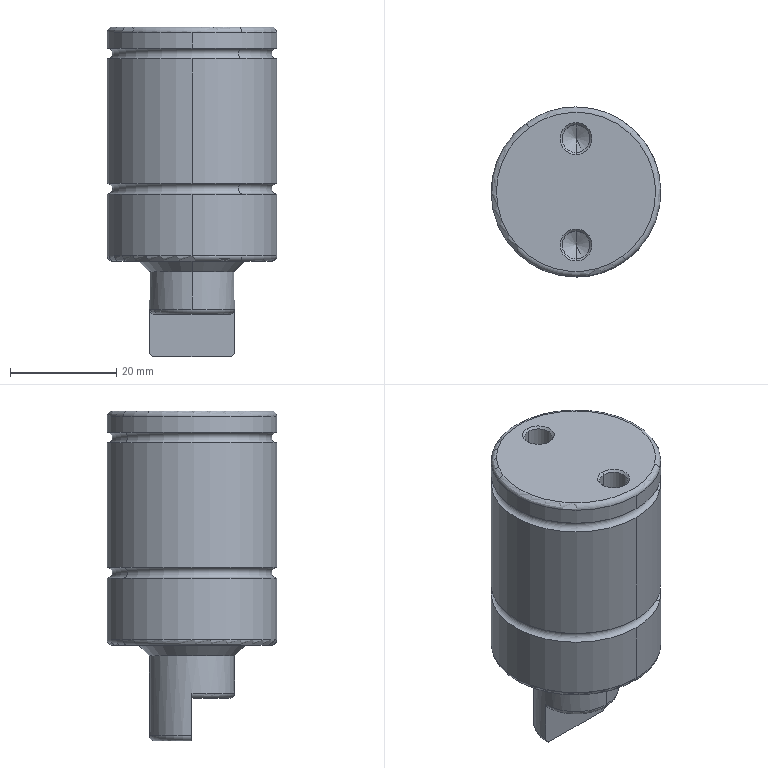Part | 1 solid | 37 faces | box 31.9 x 31.9 x 62 mm | volume 37196 mm3 | cylinder 12 | torus 10 | cone 10 | plane 5 | commonest cylinder face diameters 31.9 x6 5.2 x4 16 x2